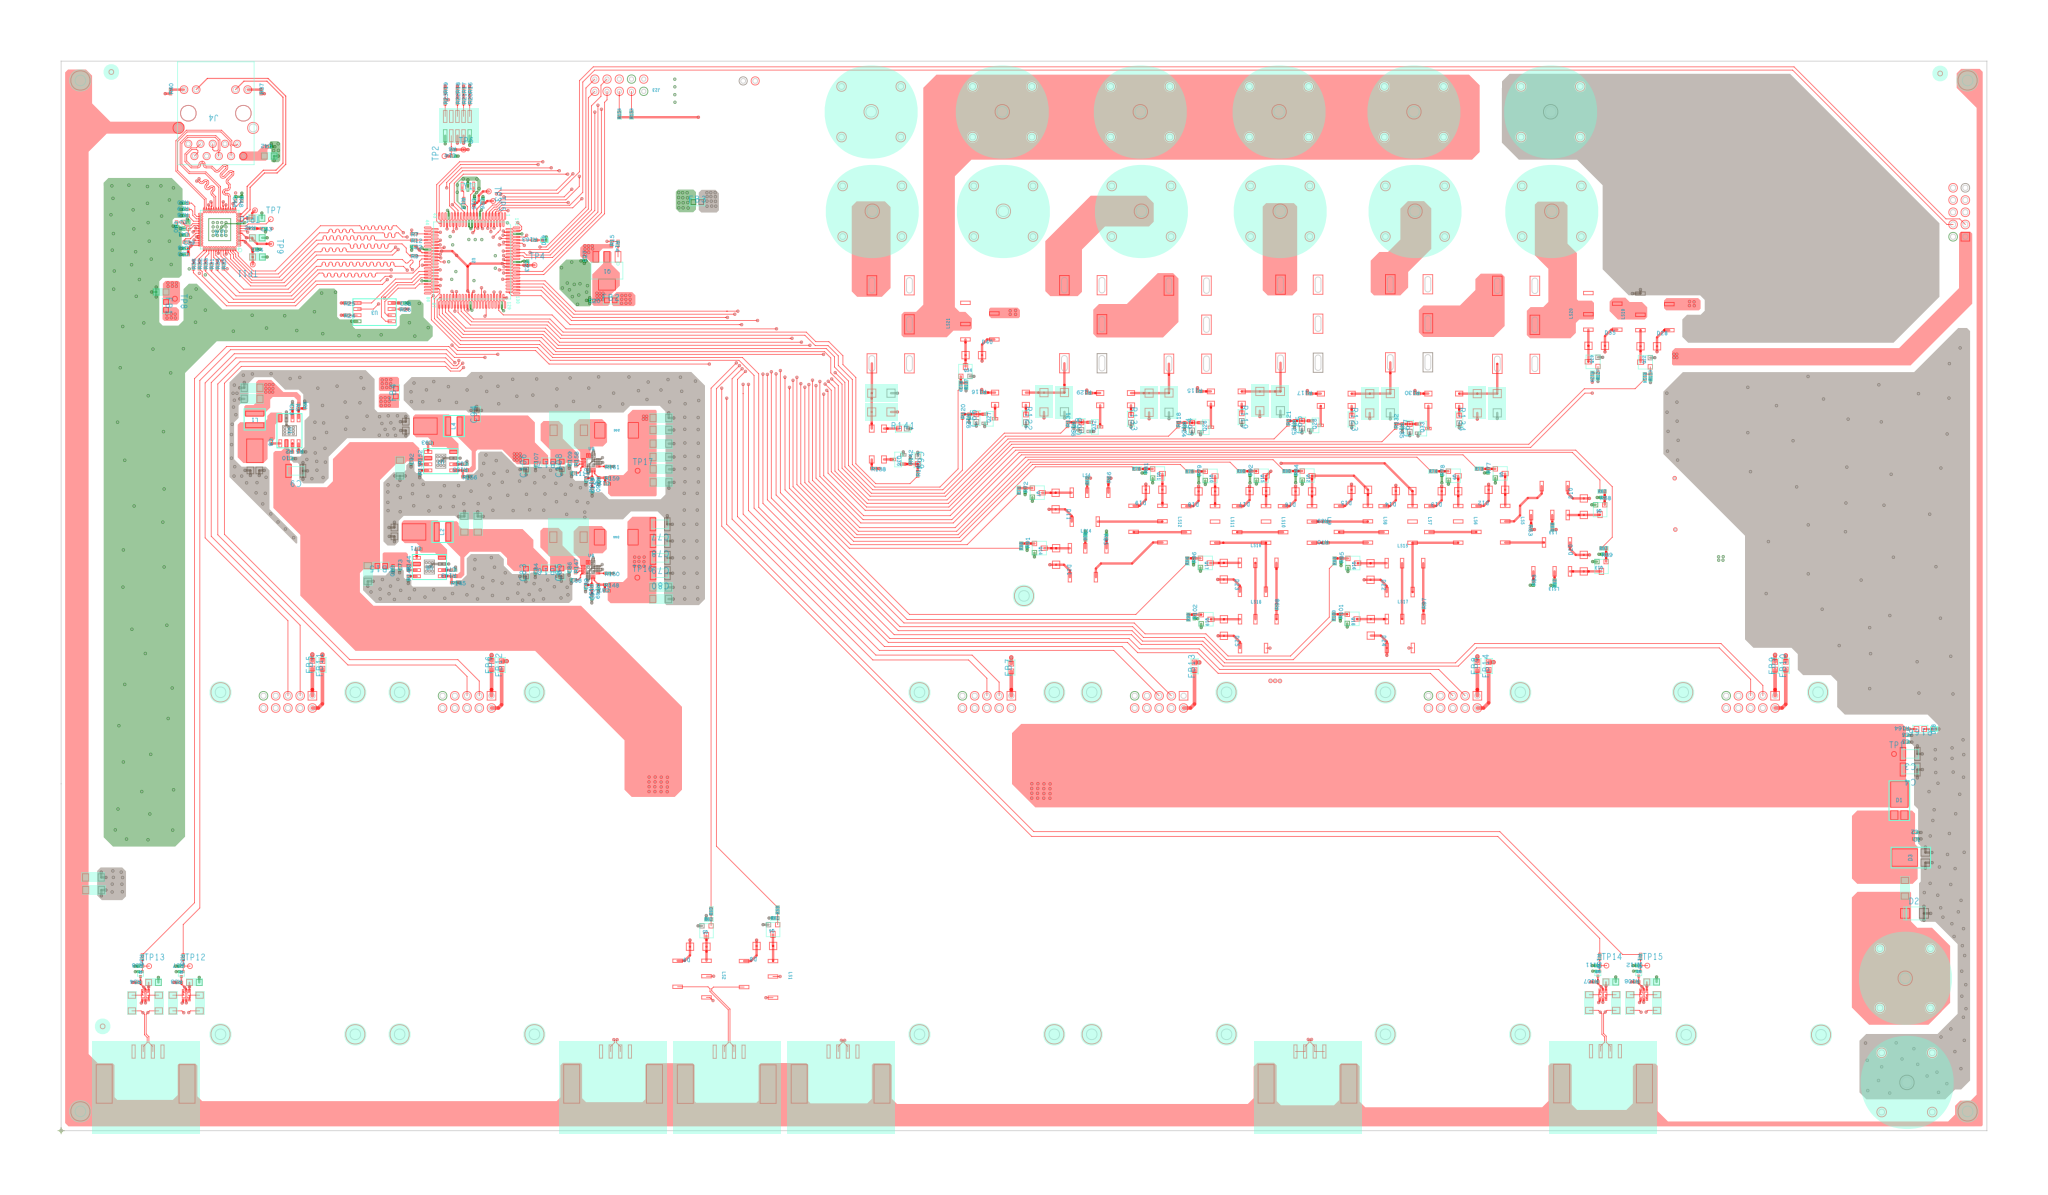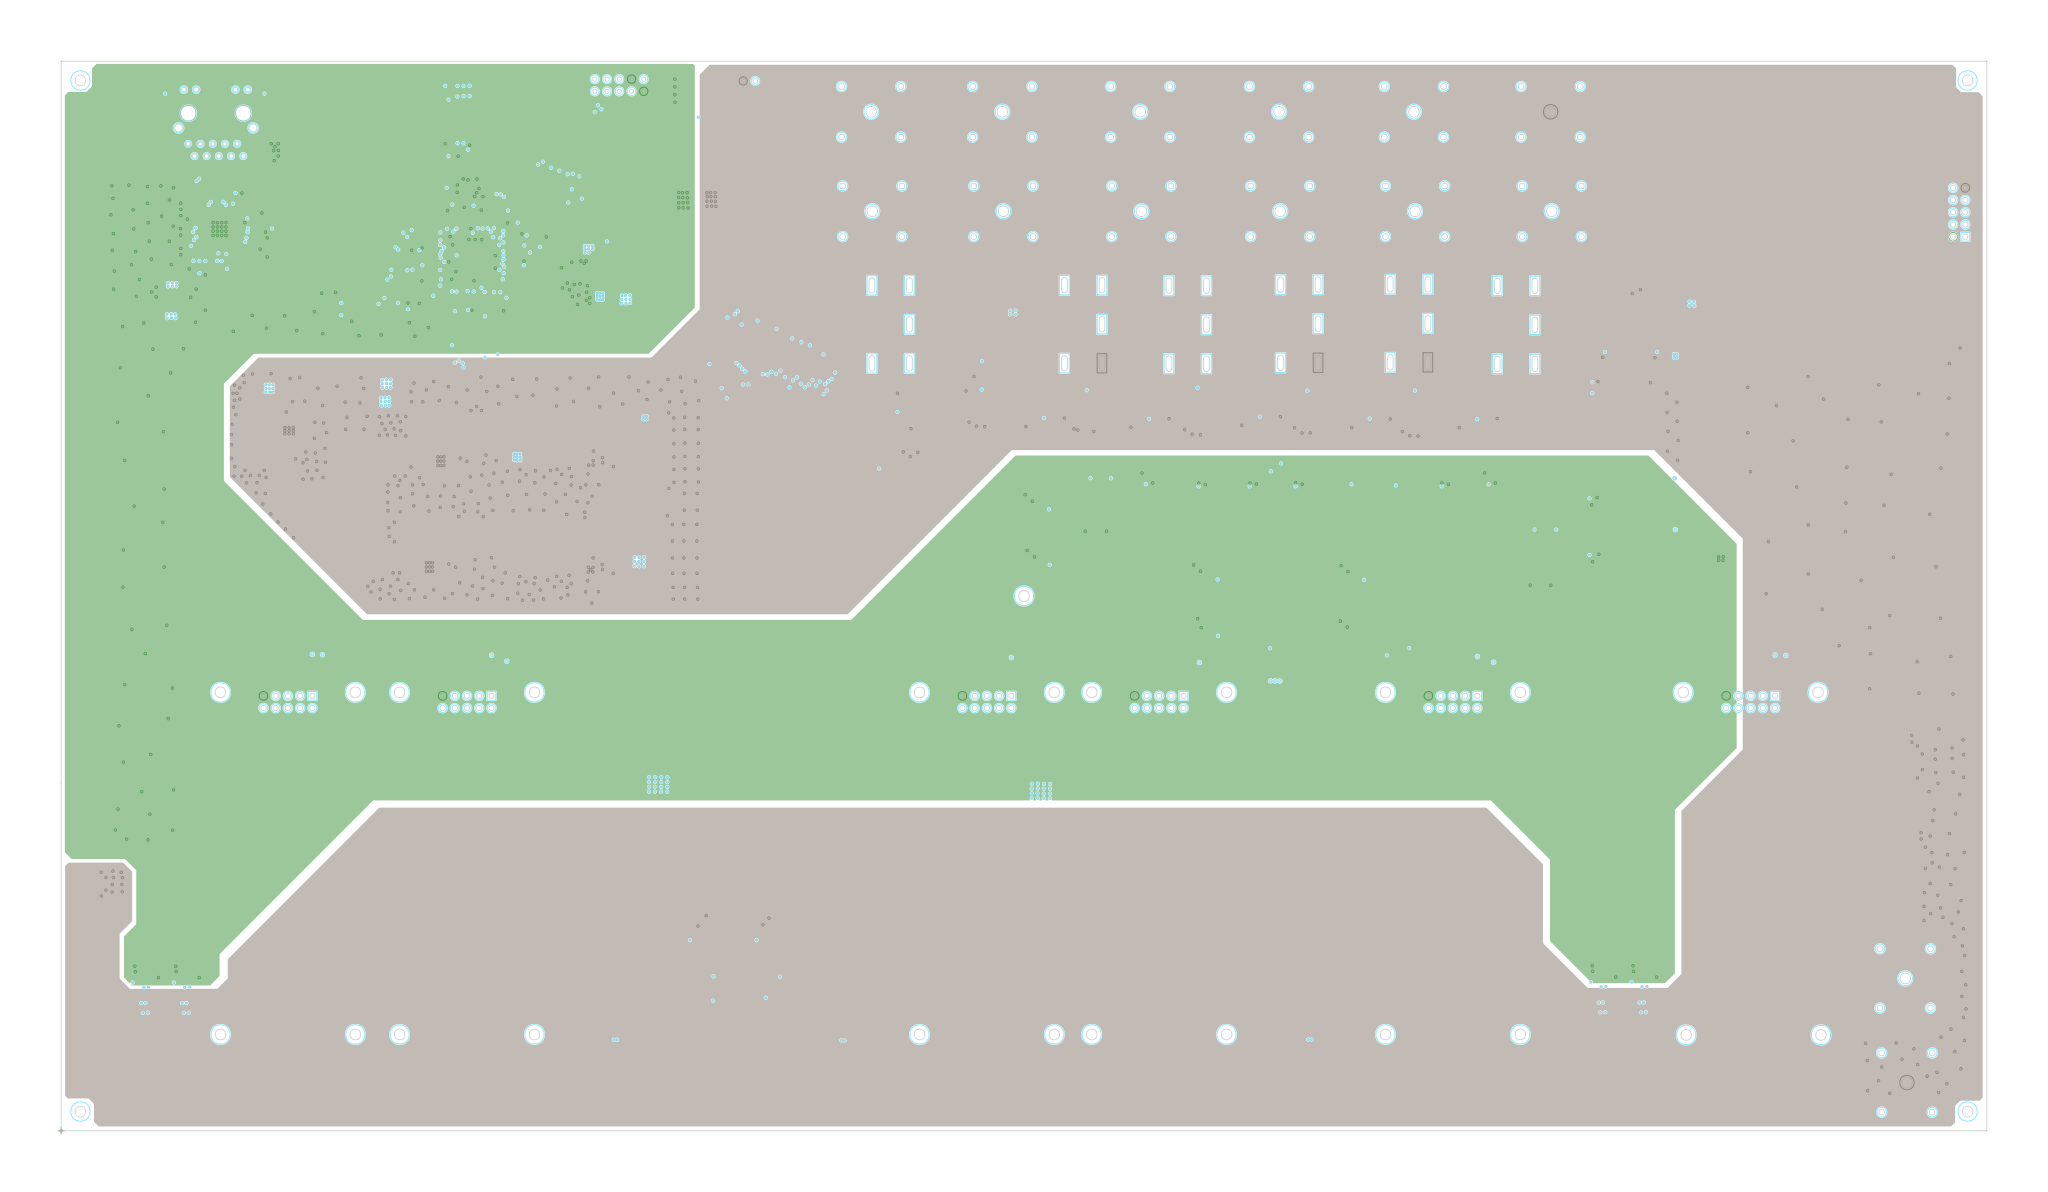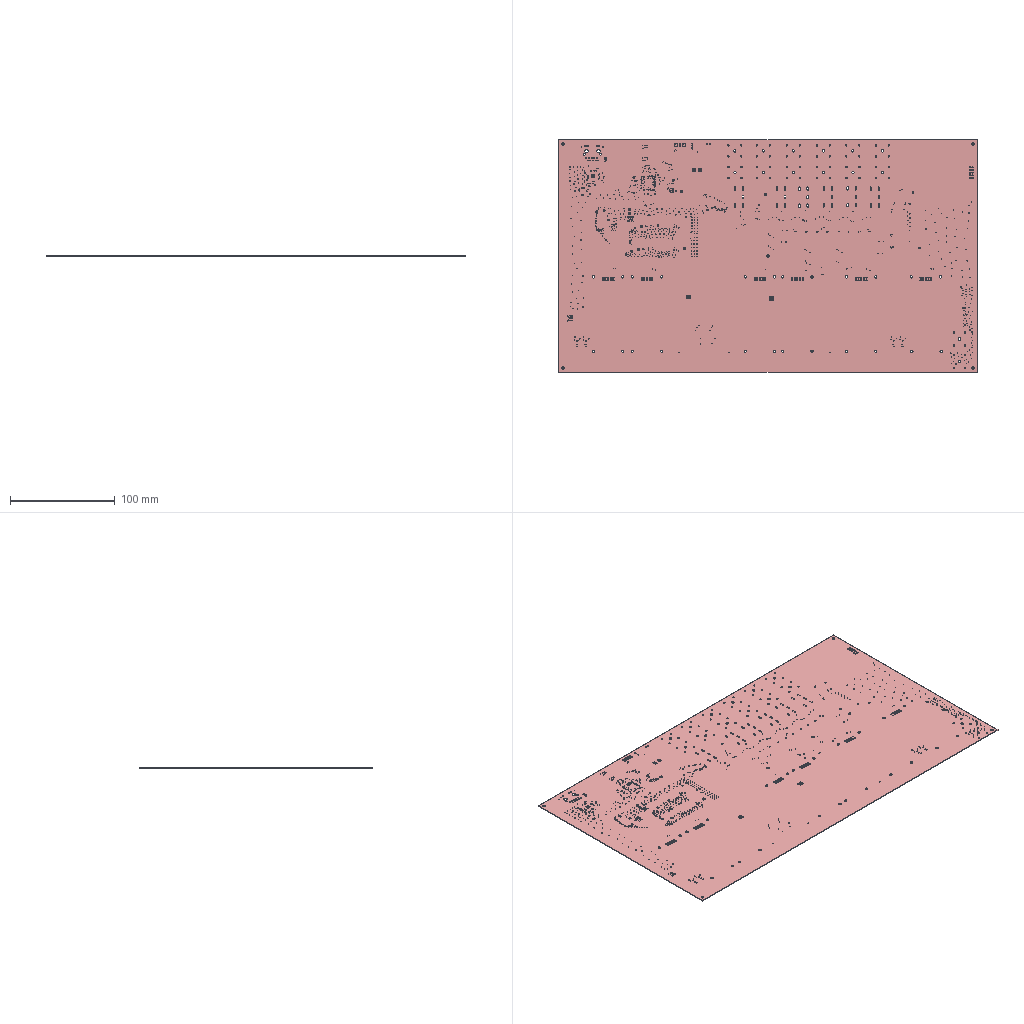Circuit board layout | Cadence Allegro | box 400 x 222 x 0.7 mm
Layer stack:
# Cadence Allegro layer stack of  (unit mm; from the constraint file cross-section; dielectric type: 0 not recorded (Allegro does not mark core vs prepreg), 3 surface material)
index,name,kind,layer,copper_thickness_mm,dielectric_type,dielectric_thickness_mm,dielectric_material,dielectric_constant
0,Top Surface,other,,,,,,
1,TOP,copper,TOP,0.0305,,,,
2,Dielectric1,dielectric,,,0,0.2032,FR-4,4.5
3,GND,copper,GND,0.0305,,,,
4,Dielectric2,dielectric,,,0,0.2032,FR-4,4.5
5,POWER,copper,POWER,0.0305,,,,
6,Dielectric3,dielectric,,,0,0.2032,FR-4,4.5
7,BOTTOM,copper,BOTTOM,0.0305,,,,
8,Bottom Surface,other,,,,,,
# drill layer pairs: low layer,high layer
drill_pair,TOP,BOTTOM
Part placement:
REFDES,COMP_VALUE,SYM_NAME,SYM_X,SYM_Y,SYM_ROTATE,SYM_MIRROR
C1,0.1uF,0402,15166.367,2384.239,0.000,NO
C2,1nF,0402,15166.922,2436.818,180.000,NO
C3,10uF_50V,1210,15121.023,3078.893,180.000,NO
C4,10uF_50V,1210,15121.082,2951.196,180.000,NO
C5,0.1uF,0402,15093.020,3175.308,180.000,NO
C6,0.1uF,0402,15092.303,3230.529,180.000,NO
C7,1nF_2kv,1206,264.027,2069.329,180.000,NO
C8,0.1uF,0402,1719.920,5633.244,270.000,NO
C9,4.7uF_50V,1210,1918.656,5392.020,180.000,NO
C10,0.1uF,0402,1876.644,5491.548,180.000,NO
C11,100uF_6.3V,1206,1561.850,6070.996,180.000,NO
C12,100uF_6.3V,1206,1561.850,5980.248,180.000,NO
C13,470pF,0402,1891.803,5916.799,270.000,NO
C14,0.1uF,0402,3207.680,7964.386,180.000,NO
C15,0.1uF,0402,3380.408,7598.514,270.000,NO
C16,0.1uF,0402,3152.512,7135.882,0.000,YES
C17,10uF_6.3V,0402,3324.539,6901.500,90.000,YES
C18,0.1uF,0402,3567.315,7076.476,180.000,YES
C19,0.1uF,0402,3152.744,7187.449,0.000,YES
C20,2.2uF_10V,0402,4339.004,6785.480,0.000,NO
C21,10uF_6.3V,0402,3335.079,6748.189,0.000,YES
C22,0.1uF,0402,2882.858,7226.445,0.000,NO
C23,0.1uF,0402,3814.416,7089.057,270.000,NO
C24,0.1uF,0402,3386.374,7322.535,270.000,YES
C25,0.1uF,0402,3333.787,7322.354,270.000,YES
C26,0.22uF_10V,0402,3449.655,7599.047,270.000,NO
C27,2.2uF_10V,0402,4278.176,7124.640,90.000,NO
C28,10uF 10V,0603,3168.937,7020.850,0.000,YES
C29,0.1uF,0402,3439.890,7324.008,270.000,YES
C30,0.1uF,0402,3627.398,7402.335,90.000,YES
C31,0.1uF,0402,3412.835,7432.705,90.000,YES
C32,0.1uF,0402,3153.031,7239.307,0.000,YES
C33,0.1uF,0402,3376.043,6902.587,90.000,YES
C34,0.1uF,0402,3567.205,7126.173,180.000,YES
C35,0.1uF,0402,3633.000,6763.000,270.000,YES
C36,0.1uF,0402,3153.795,6957.039,0.000,YES
C37,0.1uF,0402,3156.909,7323.500,270.000,YES
C38,0.1uF,0402,2792.173,6764.170,0.000,NO
C39,0.22uF,0402,1022.477,7261.467,0.000,NO
C40,6pF_1%,0402,943.650,7408.633,270.000,NO
C41,6pF_1%,0402,1022.803,7319.000,180.000,NO
C42,0.1uF,0402,1702.362,8041.280,180.000,NO
C43,47pF,0402,1654.564,7372.408,0.000,NO
C44,0.1uF,0402,1426.769,7614.459,270.000,NO
C45,0.1uF,0402,1443.836,7455.711,0.000,YES
C46,0.1uF,0402,1310.844,7507.601,90.000,YES
C47,0.1uF,0402,1237.922,7507.499,90.000,YES
C48,0.1uF,0402,1023.627,7208.982,180.000,NO
C49,0.1uF,0402,1155.950,7250.381,180.000,YES
C50,0.1uF,0402,1023.312,7159.380,180.000,NO
C51,0.1uF,0402,1287.103,7223.058,270.000,YES
C52,0.1uF,0402,1156.115,7347.444,180.000,YES
C53,0.1uF,0402,1345.635,7223.436,270.000,YES
C54,0.1uF,0402,1582.247,7203.564,0.000,NO
C55,0.1uF,0402,1436.119,7275.046,0.000,YES
C56,0.1uF,0402,1190.576,7507.830,90.000,YES
C57,0.1uF,0402,1156.576,7299.141,180.000,YES
C58,0.1uF,0402,1156.414,7396.361,180.000,YES
C59,0.1uF,0402,1359.395,7507.219,90.000,YES
C60,0.22uF 100V,0805,1089.356,1211.128,180.000,NO
C61,0.22uF 100V,0805,755.356,1211.128,180.000,NO
C62,0.22uF 100V,0805,12673.260,1215.236,180.000,NO
C63,0.22uF 100V,0805,13007.260,1215.236,180.000,NO
C64,2.2nF_50V,0603,9248.689,5753.737,90.000,NO
C65,2.2nF_50V,0603,10147.644,5769.551,90.000,NO
C66,2.2nF_50V,0603,7484.486,5823.367,90.000,NO
C67,2.2nF_50V,0603,11028.888,5743.297,90.000,NO
C68,2.2nF_50V,0603,8343.440,5757.279,90.000,NO
C69,2.2nF_50V,0603,7004.927,5479.234,270.000,NO
C70,1uF,0402,2714.401,4599.026,270.000,NO
C71,0.1uF,0402,2923.944,4752.892,180.000,NO
C72,10uF_50V,1206,2507.630,4553.368,90.000,NO
C73,0.1uF,0402,2768.099,4599.246,90.000,NO
C74,100uF_6.3V,1206,3406.840,4955.664,90.000,NO
C75,100uF_6.3V,1206,3297.656,4955.664,90.000,NO
C76,470pF,0402,3208.872,4581.288,180.000,NO
C77,4.7uF_50V,1210,4898.112,4955.552,180.000,NO
C78,4.7uF_50V,1210,4898.984,4818.957,180.000,NO
C79,4.7uF_50V,1210,4899.236,4681.124,180.000,NO
C80,4.7uF_50V,1210,4899.661,4555.730,180.000,NO
C81,10uF_50V,1206,4902.753,4439.805,180.000,NO
C82,10uF_50V,1206,4902.745,4344.734,180.000,NO
C83,10uF_16V,0603,3800.648,4560.868,90.000,NO
C84,0.1uF,0402,3877.016,4567.308,90.000,NO
C85,10uF_16V,0603,4090.788,4562.712,90.000,NO
C86,0.1uF,0402,4153.354,4577.976,90.000,NO
C87,20pF_25V,0402,4463.125,4411.714,180.000,NO
C88,47nF_10V,0402,4187.496,4501.654,0.000,NO
C89,100pF_16V,0402,4288.543,4443.821,90.000,NO
C90,0.1uF,0402,4339.653,4357.482,90.000,NO
C91,4.7uF_50V,1206,2770.610,5414.732,90.000,NO
C92,0.1uF,0402,2861.335,5464.146,90.000,NO
C93,0.1uF,0402,3017.180,5617.792,180.000,NO
C94,10uF_16V,0603,3398.560,5854.548,90.000,NO
C95,470pF,0402,3302.108,5446.188,180.000,NO
C96,10uF/25V,C0603,4955.605,8404.371,180.000,YES
C97,10uF/25V,C0603,4955.156,8466.548,180.000,YES
C98,10uF/25V,C0603,4955.416,8530.662,180.000,YES
C99,10uF/25V,C0603,4955.935,8592.840,180.000,YES
C100,4.7uF_50V,1206,4904.544,5614.512,180.000,NO
C101,4.7uF_50V,1206,4905.772,5404.728,180.000,NO
C102,4.7uF_50V,1206,4905.772,5297.996,180.000,NO
C103,4.7uF_50V,1206,4904.544,5824.300,180.000,NO
C104,10uF_50V,1206,4904.544,5726.152,180.000,NO
C105,10uF_50V,1206,4904.544,5505.328,180.000,NO
C106,10uF_16V,0603,3803.096,5434.360,90.000,NO
C107,0.1uF,0402,3879.464,5440.800,90.000,NO
C108,10uF_16V,0603,4093.236,5436.204,90.000,NO
C109,0.1uF,0402,4155.802,5451.468,90.000,NO
C110,20pF_25V,0402,4465.573,5285.206,180.000,NO
C111,47nF_10V,0402,4189.944,5375.146,0.000,NO
C112,100pF_16V,0402,4290.991,5317.313,90.000,NO
C113,0.1uF,0402,4342.101,5230.974,90.000,NO
CB1,22uF_10V,0805,1701.835,7964.729,0.000,NO
CB2,22uF_10V,0805,817.585,6853.851,180.000,NO
CB3,22uF_10V,0805,1603.878,7296.944,0.000,NO
CB4,22uF_10V,0805,1601.504,7456.003,0.000,NO
CB5,22uF_10V,0805,1605.773,7139.886,0.000,NO
D1,SL1045,TO277_65X40_H120,15032.464,2697.240,0.000,NO
D2,SMAJ36CA,SMAJ36,15156.630,1775.495,0.000,NO
D3,SL1045,TO277_65X40_H120,15126.394,2231.633,90.000,NO
D4,PDS760-13,PDS760,1584.004,5475.913,270.000,NO
D6,CSD87502Q2,DFN-6_2X2,1023.717,1107.114,0.000,NO
D7,CSD87502Q2,DFN-6_2X2,689.717,1107.114,0.000,NO
D8,DL4148,MINIMELF,5822.295,1509.303,180.000,NO
D9,DL4148,MINIMELF,5277.642,1503.358,180.000,NO
D10,DL4148,MINIMELF,12452.219,5031.852,90.000,NO
D11,DL4148,MINIMELF,8132.712,5212.978,270.000,NO
D12,DL4148,MINIMELF,11808.637,5237.525,180.000,NO
D13,DL4148,MINIMELF,11425.105,5225.482,180.000,NO
D14,DL4148,MINIMELF,11050.042,5226.998,180.000,NO
D15,DL4148,MINIMELF,10687.282,5237.297,180.000,NO
D16,DL4148,MINIMELF,10229.664,5224.022,180.000,NO
D17,DL4148,MINIMELF,9853.951,5226.352,180.000,NO
D18,DL4148,MINIMELF,9436.778,5224.337,180.000,NO
D19,DL4148,MINIMELF,9005.653,5238.073,180.000,NO
D20,DL4148,MINIMELF,12451.751,4570.325,90.000,NO
D21,DL4148,MINIMELF,8136.566,4759.915,270.000,NO
D22,DL4148,MINIMELF,10707.999,4637.018,270.000,NO
D23,DL4148,MINIMELF,9507.692,4639.569,270.000,NO
D24,DL4148,MINIMELF,10710.053,4180.729,270.000,NO
D25,DL4148,MINIMELF,9508.715,4179.032,270.000,NO
D26,CSD87502Q2,DFN-6_2X2,12607.621,1111.222,0.000,NO
D27,CSD87502Q2,DFN-6_2X2,12941.621,1111.222,0.000,NO
D28,DL4148,MINIMELF,12915.801,6410.084,0.000,NO
D29,SMAJ16A,DO-214AC,9970.841,5962.570,90.000,NO
D30,SMAJ16A,DO-214AC,9802.731,5962.300,270.000,NO
D31,SMAJ16A,DO-214AC,8205.008,5953.394,90.000,NO
D32,SMAJ16A,DO-214AC,8037.507,5952.516,270.000,NO
D33,SMAJ16A,DO-214AC,10869.900,5944.831,90.000,NO
D34,SMAJ16A,DO-214AC,10701.790,5943.953,270.000,NO
D35,DL4148,MINIMELF,12490.078,6414.102,0.000,NO
D36,SMAJ16A,DO-214AC,9059.747,5949.575,90.000,NO
D37,SMAJ16A,DO-214AC,8897.082,5948.698,270.000,NO
D38,SMAJ16A,DO-214AC,11744.154,5944.629,90.000,NO
D39,SMAJ16A,DO-214AC,11580.889,5944.359,270.000,NO
D40,DL4148,MINIMELF,7396.079,6337.715,0.000,NO
D41,SMAJ16A,DO-214AC,6707.776,6026.964,180.000,NO
D42,SMAJ16A,DO-214AC,6707.179,5873.400,0.000,NO
D43,PDS760-13,PDS760,2805.583,4892.934,180.000,NO
D44,B540C-13-F,SMC,4539.783,4849.992,180.000,NO
D45,PDS760-13,PDS760,2898.819,5757.834,180.000,NO
D46,B540C-13-F,SMC,4542.231,5723.484,180.000,NO
D48,NCD0402R1,LED0402_H050,15316.437,3282.242,90.000,NO
D49,NCD0402G1,LED0402_H050,3951.797,7277.576,90.000,NO
F1,Fuse_5A,1206,15077.756,1980.860,90.000,NO
FB1,BLM18KG300TN1D,0603,857.870,6740.076,270.000,NO
FB2,BLM18KG300TN1D,0603,4494.897,6785.278,0.000,NO
FB3,BLM18KG300TN1D,0603,5202.406,7588.192,0.000,NO
FB4,BLM18KG300TN1D,0603,2736.804,6032.536,90.000,NO
FB5,BLM18KG300TN1D,0603,2054.449,3807.862,90.000,NO
FB6,BLM18KG300TN1D,0603,3520.103,3805.863,90.000,NO
FB7,BLM18KG300TN1D,0603,7770.126,3784.850,90.000,NO
FB8,BLM18KG300TN1D,0603,11581.861,3797.677,90.000,NO
FB9,BLM18KG300TN1D,0603,14016.188,3799.077,90.000,NO
FB10,BLM18KG300TN1D,0603,14103.578,3799.739,90.000,NO
FB11,BLM18KG300TN1D,0603,2136.902,3806.469,90.000,NO
FB12,BLM18KG300TN1D,0603,3602.449,3805.256,90.000,NO
FB13,BLM18KG300TN1D,0603,9268.598,3795.001,90.000,NO
FB14,BLM18KG300TN1D,0603,11674.222,3796.973,90.000,NO
FB15,BLM18KG300TN1D,0603,2618.169,4615.868,180.000,NO
FB16,BLM18KG300TN1D,0603,3990.028,4594.500,180.000,NO
FB17,BLM18KG300TN1D,0603,3992.476,5467.992,180.000,NO
J1,4mm_Angled_Socket,YJX40016A,15080.346,1245.134,90.000,NO
J2,4mm_Angled_Socket,YJX40016A,15094.453,394.134,90.000,NO
J3,HB-PH9-12725PB2GOB,JTAG_2X5_1P27MM,3240.811,8209.965,180.000,NO
J4,HR915330AE,HR915330AE,1265.142,8314.736,180.000,NO
J5,BH254V-10P,BH254V-10P,1854.654,3503.909,180.000,NO
J6,4mm_Angled_Socket,YJX40016A,8825.083,8326.665,0.000,NO
J7,4mm_Angled_Socket,YJX40016A,8834.205,7513.695,0.000,NO
J8,BH254V-10P,BH254V-10P,3319.386,3503.909,180.000,NO
J9,349128040,349128040,4513.622,514.280,0.000,NO
J10,349128040,349128040,6374.303,514.280,0.000,NO
J11,349128040,349128040,5443.059,512.760,0.000,NO
J12,BH254V-10P,BH254V-10P,7570.622,3503.913,180.000,NO
J13,BH254V-10P,BH254V-10P,8979.106,3503.909,180.000,NO
J14,349128040,349128040,10192.319,514.567,0.000,NO
J15,4mm_Angled_Socket,YJX40016A,9960.028,8326.665,0.000,NO
J16,4mm_Angled_Socket,YJX40016A,9969.150,7513.691,0.000,NO
J17,4mm_Angled_Socket,YJX40016A,6633.248,7513.695,0.000,NO
J18,4mm_Angled_Socket,YJX40016A,6624.130,8326.661,0.000,NO
J19,BH254V-10P,BH254V-10P,11381.370,3503.909,180.000,NO
J20,4mm_Angled_Socket,YJX40016A,12189.957,7513.695,0.000,NO
J21,4mm_Angled_Socket,YJX40016A,12180.835,8326.665,0.000,NO
J22,B2B-XH-A,B2B-XH-A,5626.740,8578.846,0.000,NO
J23,BH2x5P_2.54,BH2X5P_2_54,4564.335,8543.811,180.000,NO
J25,BH254V-10P,BH254V-10P,15521.988,7505.402,90.000,NO
J26,4mm_Angled_Socket,YJX40016A,11062.811,8326.665,0.000,NO
J27,4mm_Angled_Socket,YJX40016A,11071.933,7513.695,0.000,NO
J28,4mm_Angled_Socket,YJX40016A,7696.409,8326.665,0.000,NO
J29,4mm_Angled_Socket,YJX40016A,7705.535,7513.691,0.000,NO
J30,BH254V-10P,BH254V-10P,13816.256,3504.157,180.000,NO
J31,349128040,349128040,690.921,513.929,0.000,NO
J32,349128040,349128040,12609.244,516.886,0.000,NO
L1,FEXL0430A-2R2M,L_41X41_H210_BOURNS,1583.098,5812.295,180.000,NO
L2,FEXL0430A-2R2M,L_41X41_H210_BOURNS,3119.072,4893.178,90.000,NO
L3,SLF7045T100M,SMD_7X7,4148.803,4850.437,0.000,NO
L4,FEXL0430A-2R2M,L_41X41_H210_BOURNS,3212.308,5758.078,90.000,NO
L5,SLF7045T100M,SMD_7X7,4151.251,5723.929,0.000,NO
LS1,IMC03GR,IMC03GR,5585.075,1385.996,270.000,NO
LS2,IMC03GR,IMC03GR,5041.327,1388.331,270.000,NO
LS3,IMC03GR,IMC03GR,12320.353,5267.360,180.000,NO
LS4,IMC03GR,IMC03GR,8264.574,4977.470,0.000,NO
LS5,IMC03GR,IMC03GR,11573.129,5105.663,270.000,NO
LS6,IMC03GR,IMC03GR,11188.653,5104.675,270.000,NO
LS7,IMC03GR,IMC03GR,10815.278,5103.793,270.000,NO
LS8,IMC03GR,IMC03GR,10449.810,5105.474,270.000,NO
LS9,IMC03GR,IMC03GR,9993.027,5103.514,270.000,NO
LS10,IMC03GR,IMC03GR,9617.235,5103.825,270.000,NO
LS11,IMC03GR,IMC03GR,9200.322,5103.529,270.000,NO
LS12,IMC03GR,IMC03GR,8770.145,5106.207,270.000,NO
LS13,IMC03GR,IMC03GR,12339.038,4806.951,180.000,NO
LS14,IMC03GR,IMC03GR,8249.278,4523.289,0.000,NO
LS15,IMC03GR,IMC03GR,10839.861,4401.510,0.000,NO
LS16,IMC03GR,IMC03GR,9639.554,4404.061,0.000,NO
LS17,IMC03GR,IMC03GR,10841.312,3944.617,0.000,NO
LS18,IMC03GR,IMC03GR,9640.582,3943.524,0.000,NO
LS19,IMC03GR,IMC03GR,13151.305,6541.950,90.000,NO
LS20,IMC03GR,IMC03GR,12725.582,6545.968,90.000,NO
LS21,IMC03GR,IMC03GR,7631.476,6466.035,90.000,NO
MH1,MOUNTING_HOLE,HOLE2_2_4,15590.551,157.480,0.000,NO
MH2,MOUNTING_HOLE,HOLE2_2_4,15590.551,8582.677,0.000,NO
MH3,MOUNTING_HOLE,HOLE2_2_4,157.480,8582.677,0.000,NO
MH4,MOUNTING_HOLE,HOLE2_2_4,157.480,157.480,0.000,NO
Q1,BCP56-16TX,BCP56_SOT-223,4463.479,7028.459,180.000,NO
Q2,CJ3134K KF,SOT723,982.913,1279.720,180.000,NO
Q3,CJ3134K KF,SOT723,648.913,1279.720,180.000,NO
Q4,NDS331N,SOT23-3,5859.484,1683.398,180.000,NO
Q5,NDS331N,SOT23-3,5315.217,1673.791,180.000,NO
Q6,NDS331N,SOT23-3,12623.058,5115.033,180.000,NO
Q7,NDS331N,SOT23-3,7942.499,5251.514,270.000,NO
Q8,NDS331N,SOT23-3,11728.496,5408.368,270.000,NO
Q9,NDS331N,SOT23-3,11344.920,5389.199,270.000,NO
Q10,NDS331N,SOT23-3,9356.590,5388.053,270.000,NO
Q11,NDS331N,SOT23-3,8926.119,5407.695,270.000,NO
Q12,NDS331N,SOT23-3,10149.223,5390.561,270.000,NO
Q13,NDS331N,SOT23-3,12634.428,4650.640,180.000,NO
Q14,NDS331N,SOT23-3,7959.507,4798.399,270.000,NO
Q15,NDS331N,SOT23-3,9774.514,5388.915,270.000,NO
Q16,NDS331N,SOT23-3,10522.987,4676.372,270.000,NO
Q17,NDS331N,SOT23-3,9317.095,4677.200,270.000,NO
Q18,NDS331N,SOT23-3,10517.317,4220.043,270.000,NO
Q19,NDS331N,SOT23-3,9323.222,4216.835,270.000,NO
Q20,CJ3134K KF,SOT723,12566.817,1283.828,180.000,NO
Q21,CJ3134K KF,SOT723,12900.817,1283.828,180.000,NO
Q22,NDS331N,SOT23-3,12995.823,6242.406,90.000,NO
Q23,TLP187,TLP187,9528.613,5991.528,270.000,NO
Q24,TLP187,TLP187,7763.389,5981.745,270.000,NO
Q25,TLP187,TLP187,10427.672,5973.186,270.000,NO
Q26,BSS138,003_SOT23B,9317.526,5786.151,0.000,NO
Q27,BSS138,003_SOT23B,7552.218,5855.229,0.000,NO
Q28,BSS138,003_SOT23B,10215.372,5801.409,0.000,NO
Q29,NDS331N,SOT23-3,12567.995,6245.367,90.000,NO
Q30,TLP187,TLP187,8622.960,5977.922,270.000,NO
Q31,TLP187,TLP187,11306.771,5973.587,270.000,NO
Q32,BSS138,003_SOT23B,8411.172,5789.137,0.000,NO
Q33,BSS138,003_SOT23B,11096.616,5775.159,0.000,NO
Q34,NDS331N,SOT23-3,7357.592,6164.352,0.000,NO
Q35,TLP187,TLP187,6678.996,5611.430,0.000,NO
Q36,BSS138,003_SOT23B,6886.936,5447.585,180.000,NO
R1,1M,1206,264.991,1966.310,0.000,NO
R2,100K,0402,1875.106,5545.811,180.000,NO
R3,51K,0402,1941.669,5918.819,270.000,NO
R4,15K,0402,1991.559,5918.898,90.000,NO
R5,20K,0402,1958.909,5546.988,180.000,NO
R6,4.7K,0402,3207.434,8017.034,180.000,NO
R7,33R,0402,2883.035,7329.154,0.000,NO
R8,33R,0402,2883.000,7328.744,180.000,YES
R9,33R,0402,2882.492,7150.524,0.000,NO
R10,33R,0402,2884.272,7226.547,180.000,YES
R11,33R,0402,2882.138,7276.886,180.000,YES
R12,33R,0402,2883.201,7277.307,0.000,NO
R13,0R,0402,3292.260,7600.390,270.000,NO
R14,10K,0402,4554.378,7250.672,270.000,NO
R15,2.2K,0402,4500.280,7251.105,90.000,NO
R16,4.7K,0402,3340.905,8498.590,90.000,NO
R17,4.7K,0402,3291.038,8498.717,90.000,NO
R18,4.7K,0402,3240.439,8499.024,90.000,NO
R19,4.7K,0402,3140.528,8498.881,90.000,NO
R20,33R,0402,3340.884,8410.028,90.000,NO
R21,33R,0402,3291.335,8410.146,90.000,NO
R22,33R,0402,3240.626,8409.941,90.000,NO
R23,33R,0402,3140.496,8408.717,90.000,NO
R24,4.7K,0402,2334.673,6664.475,0.000,NO
R25,4.7K,0402,2334.482,6764.138,0.000,NO
R26,10K,0402,2791.985,6714.205,0.000,NO
R28,49R9,0402,1020.036,7477.723,180.000,NO
R29,49R9,0402,1020.202,7528.956,180.000,NO
R30,4.99K,0402,1020.583,7580.066,180.000,NO
R31,33R,0402,1227.553,7060.363,90.000,NO
R32,33R,0402,1130.313,7060.422,90.000,NO
R33,33R,0402,1179.400,7060.682,90.000,NO
R34,33R,0402,1276.837,7060.607,90.000,NO
R35,33R,0402,1326.474,7060.576,90.000,NO
R36,33R,0402,1081.679,7059.190,90.000,NO
R37,510R,0402,1635.395,8490.854,90.000,NO
R38,4.7K,0402,1568.780,7318.235,180.000,YES
R39,4.7K,0402,1569.079,7372.668,180.000,YES
R40,510R,0402,894.325,8491.276,90.000,NO
R41,4.7K,0402,1426.773,7614.424,270.000,YES
R42,49R9,0402,1569.485,7372.570,180.000,NO
R43,4.7K,0402,1081.317,7059.182,270.000,YES
R44,4.7K,0402,1130.474,7060.154,270.000,YES
R45,4.7K,0402,1326.581,7060.257,270.000,YES
R46,4.7K,0402,1276.278,7060.650,270.000,YES
R47,4.7K,0402,1179.108,7060.871,270.000,YES
R48,4.7K,0402,1477.757,7615.255,270.000,NO
R49,49R9  0.4W 1206,1206,1132.583,1043.043,90.000,NO
R50,49R9  0.4W 1206,1206,912.640,1042.945,90.000,NO
R51,49R9  0.4W 1206,1206,798.583,1043.043,90.000,NO
R52,49R9  0.4W 1206,1206,578.640,1042.945,90.000,NO
R53,10K,0402,966.725,1211.525,180.000,NO
R54,10K,0402,632.725,1211.525,180.000,NO
R55,100R,0402,998.398,1419.035,270.000,NO
R56,100R,0402,664.398,1419.035,270.000,NO
R57,100R,0402,982.189,1344.772,180.000,NO
R58,100R,0402,648.189,1344.772,180.000,NO
R59,100R,R0402,5859.575,1804.209,90.000,NO
R60,100R,R0402,5314.965,1793.835,90.000,NO
R61,4.7K,R0402,5839.634,1737.697,0.000,NO
R62,4.7K,R0402,5295.445,1727.933,0.000,NO
R63,0R,0402,12021.161,4929.218,270.000,NO
R64,62R,R0402,12193.979,4932.179,270.000,NO
R65,62R,R0402,8390.948,5313.179,90.000,NO
R66,0R,0402,8564.554,5315.612,90.000,NO
R67,100R,R0402,12603.593,5224.651,0.000,NO
R68,4.7K,0402,12606.125,5174.466,0.000,NO
R69,1K,0402,10342.003,4977.475,180.000,NO
R70,0R,0402,10342.467,4804.407,180.000,NO
R71,100R,R0402,7832.881,5232.049,90.000,NO
R72,4.7K,0402,7883.066,5234.585,90.000,NO
R73,100R,R0402,11598.646,5408.041,0.000,NO
R74,100R,R0402,11221.754,5389.007,0.000,NO
R75,100R,R0402,9229.028,5387.262,0.000,NO
R76,100R,R0402,8794.369,5408.017,0.000,NO
R77,4.7K,0402,11668.748,5391.970,90.000,NO
R78,4.7K,0402,11291.070,5372.573,90.000,NO
R79,4.7K,0402,9302.739,5371.427,90.000,NO
R80,100R,R0402,10023.110,5390.606,0.000,NO
R81,4.7K,0402,8866.371,5391.298,90.000,NO
R82,62R,R0402,12213.184,4476.230,90.000,NO
R83,0R,0402,12039.562,4474.478,90.000,NO
R84,4.7K,0402,10095.281,5374.154,90.000,NO
R85,0R,0402,8548.751,4855.758,270.000,NO
R86,62R,R0402,8375.133,4854.006,270.000,NO
R87,100R,R0402,12614.528,4759.604,0.000,NO
R88,100R,R0402,7850.538,4779.111,90.000,NO
R89,4.7K,0402,12618.015,4710.722,0.000,NO
R90,100R,R0402,9651.812,5389.715,0.000,NO
R91,4.7K,0402,7899.424,4781.990,90.000,NO
R92,4.7K,0402,9722.104,5373.309,90.000,NO
R93,100R,R0402,10414.653,4657.417,90.000,NO
R94,100R,R0402,9208.577,4658.306,90.000,NO
R95,4.7K,0402,10466.570,4660.344,90.000,NO
R96,4.7K,0402,9260.677,4661.173,90.000,NO
R97,1K,0402,11140.799,4285.187,90.000,NO
R98,1K,0402,9938.912,4277.738,90.000,NO
R99,100R,R0402,9218.506,4197.280,90.000,NO
R100,100R,R0402,10408.191,4201.152,90.000,NO
R101,4.7K,0402,10460.904,4204.015,90.000,NO
R102,4.7K,0402,9266.805,4200.807,90.000,NO
R103,49R9  0.4W 1206,1206,12716.487,1047.151,90.000,NO
R104,49R9  0.4W 1206,1206,12496.544,1047.053,90.000,NO
R105,49R9  0.4W 1206,1206,13050.487,1047.151,90.000,NO
R106,49R9  0.4W 1206,1206,12830.544,1047.053,90.000,NO
R107,10K,0402,12550.629,1215.633,180.000,NO
R108,10K,0402,12884.629,1215.633,180.000,NO
R109,100R,0402,12582.302,1423.143,270.000,NO
R110,100R,0402,12916.302,1423.143,270.000,NO
R111,100R,0402,12566.093,1348.880,180.000,NO
R112,100R,0402,12900.093,1348.880,180.000,NO
R113,4.7K,R0402,12997.185,6162.670,90.000,NO
R114,100R,R0402,12951.488,6162.843,270.000,NO
R115,470R,0402,9309.205,6041.824,180.000,NO
R116,470R,0402,7544.996,6031.969,180.000,NO
R117,470R,0402,10207.724,6023.194,180.000,NO
R118,100R,0402,9132.945,5769.512,90.000,NO
R119,2k_0603,0603,9654.869,5831.016,270.000,NO
R120,100R,0402,7370.566,5838.838,90.000,NO
R121,100R,0402,10032.811,5784.110,90.000,NO
R122,2k_0603,0603,7889.645,5821.237,270.000,NO
R123,2k_0603,0603,10553.928,5812.674,270.000,NO
R124,4.7K,0402,9187.556,5769.572,270.000,NO
R125,4.7K,0402,10086.510,5784.473,270.000,NO
R126,4.7K,0402,7424.264,5838.593,270.000,NO
R127,4.7K,R0402,12567.868,6171.300,90.000,NO
R128,100R,R0402,12522.172,6171.477,270.000,NO
R129,470R,0402,8404.011,6027.930,180.000,NO
R130,470R,0402,11087.818,6023.711,180.000,NO
R131,100R,0402,8229.520,5772.446,90.000,NO
R132,100R,0402,10913.144,5758.768,90.000,NO
R133,2k_0603,0603,8749.216,5817.414,270.000,NO
R134,2k_0603,0603,11433.027,5813.075,270.000,NO
R135,4.7K,0402,10967.754,5758.523,270.000,NO
R136,4.7K,0402,8282.914,5772.506,270.000,NO
R137,4.7K,R0402,7400.025,6090.922,90.000,NO
R138,470R,0402,6645.516,5411.104,0.000,NO
R139,100R,R0402,7356.911,6091.222,270.000,NO
R140,100R,0402,7004.442,5366.944,90.000,NO
R141,2k_0603,0603,6883.972,5737.588,0.000,NO
R142,4.7K,0402,6943.361,5464.356,90.000,NO
R143,51.1K,0402,3209.024,4531.206,180.000,NO
R144,100K,0402,2837.764,4598.100,90.000,NO
R145,9.09K,0402,3209.811,4478.490,0.000,NO
R146,20K,0402,2838.630,4514.348,90.000,NO
R147,10K,0402,4206.496,4577.378,90.000,NO
R148,88.7K_1%,0402,4463.814,4461.785,0.000,NO
R149,10K,0402,4393.920,4445.884,270.000,NO
R150,78.7K_1%,0402,4467.036,4554.668,0.000,NO
R151,2.55K_1%,0402,4339.586,4443.899,270.000,NO
R152,100K,0402,2931.000,5463.000,90.000,NO
R153,NC,R0402,4663.897,8301.836,90.000,NO
R154,NC,R0402,4564.195,8302.122,90.000,NO
R155,51.1K,0402,3302.260,5396.106,180.000,NO
R156,9.09K,0402,3303.047,5343.390,0.000,NO
R157,20K,0402,2931.866,5379.248,90.000,NO
R158,10K_1%,0402,4208.944,5450.870,90.000,NO
R159,113K_1%,0402,4466.262,5335.277,0.000,NO
R160,10K_1%,0402,4396.368,5319.376,270.000,NO
R161,78.7K_1%,0402,4469.484,5428.160,0.000,NO
R162,2.55K_1%,0402,4342.034,5317.391,270.000,NO
R163,1.8K,0402,3870.315,7277.630,180.000,NO
R164,1.8K,0402,15092.597,3282.701,180.000,NO
R166,2k_0603,0603,15203.882,3282.513,180.000,NO
RY1,HFV9-012-1ZR,HFV9-012-1ZR,10125.361,6594.811,270.000,NO
RY2,HFV9-012-1ZR,HFV9-012-1ZR,8357.901,6590.520,270.000,NO
RY3,HFV9-012-1ZR,HFV9-012-1ZR,11023.161,6598.126,270.000,NO
RY4,HFV9-012-1ZR,HFV9-012-1ZR,9212.680,6586.929,270.000,NO
RY5,HFV9-012-1ZR,HFV9-012-1ZR,11898.141,6585.555,270.000,NO
RY6,HFV9-012-1ZR,HFV9-012-1ZR,6783.614,6589.531,270.000,NO
TP1,TP,S0400CI,14988.796,3078.372,0.000,NO
TP2,TP,S0400CI,3134.272,7964.144,90.000,NO
TP3,TP,S0400CI,3497.598,7675.665,270.000,NO
TP4,TP,S0400CI,3871.401,7073.045,0.000,NO
TP5,TP,S0400CI,3532.906,7597.425,270.000,NO
TP6,TP,S0400CI,3291.081,8017.433,0.000,NO
TP7,TP,S0400CI,1714.969,7448.700,0.000,NO
TP8,TP,S0400CI,930.452,6798.856,270.000,NO
TP9,TP,S0400CI,1717.928,7247.157,270.000,NO
TP10,TP,S0400CI,1585.260,7521.272,180.000,NO
TP11,TP,S0400CI,1566.969,7078.804,180.000,NO
TP12,TP,S0400CI,1053.614,1344.366,0.000,NO
TP13,TP,S0400CI,719.614,1344.366,0.000,NO
TP14,TP,S0400CI,12637.518,1348.474,0.000,NO
TP15,TP,S0400CI,12971.518,1348.474,0.000,NO
TP16,TP,S0400CI,4711.945,4519.469,0.000,NO
TP17,TP,S0400CI,4714.393,5392.961,0.000,NO
U1,LMR14050SQDDARQ1,SOP8P_60_PAD29X21_127_H170,1867.134,5719.744,270.000,NO
U2,S32K314EHTVBPBST_MaxQFP172,MQFP172_0P65_16X16,3360.819,7111.406,270.000,NO
U3,W25Q128JVSIQ,SO8P_79_127_H220,2563.090,6689.287,180.000,NO
U4,88EA1512_QFN56,QFN50P800X800X100-56N_180X180EP,1296.477,7363.239,180.000,NO
U5,LMR14050SQDDARQ1,SOP8P_60_PAD29X21_127_H170,3011.386,4606.124,180.000,NO
U6,TPS55340RTER,WQFN16-3X3,4270.826,4525.143,0.000,NO
U7,LMR14050SQDDARQ1,SOP8P_60_PAD29X21_127_H170,3104.622,5471.024,180.000,NO
U8,TPS55340RTER,WQFN16-3X3,4273.274,5398.635,0.000,NO
Y1,CSTNE16M0V53C000R0,CSTNE16M0V53C000R0,3326.374,7714.500,0.000,NO
Y2,XRCGB25M000F3A00R00,CRYSTAL_SM,1019.824,7398.826,90.000,NO
Pad and via stacks, first 112 of 394 lines:
# Allegro (Cadence) via spans and padstacks; design units: ("mils" 3 1000)
# via spans: padstack,start_layer,end_layer,net_example,count
VIA12X20,ETCH/TOP,ETCH/BOTTOM,BAT_GND,1173
VIA15_30,ETCH/TOP,ETCH/BOTTOM,NODE6_DUT_GND_PWR,15
# Allegro padstack definitions: name,start_layer,end_layer,drill,plating,holeType,type
PAD19,"ETCH/TOP","ETCH/TOP",0.0,"NON_PLATED","none","smd"
PAD13,"ETCH/TOP","ETCH/TOP",0.0,"NON_PLATED","none","smd"
PAD12,"ETCH/TOP","ETCH/TOP",0.0,"NON_PLATED","none","smd"
PAD17,"ETCH/TOP","ETCH/TOP",0.0,"NON_PLATED","none","smd"
PAD15,"ETCH/TOP","ETCH/TOP",0.0,"NON_PLATED","none","smd"
PAD16,"ETCH/TOP","ETCH/TOP",0.0,"NON_PLATED","none","smd"
PAD1,"ETCH/TOP","ETCH/TOP",0.0,"NON_PLATED","none","smd"
PAD46,"ETCH/TOP","ETCH/TOP",0.0,"NON_PLATED","none","smd"
PAD44,"ETCH/TOP","ETCH/TOP",0.0,"NON_PLATED","none","smd"
PAD8,"ETCH/TOP","ETCH/TOP",0.0,"NON_PLATED","none","smd"
PAD5,"ETCH/TOP","ETCH/TOP",0.0,"NON_PLATED","none","smd"
PAD9,"ETCH/TOP","ETCH/TOP",0.0,"NON_PLATED","none","smd"
PAD10,"ETCH/TOP","ETCH/TOP",0.0,"NON_PLATED","none","smd"
PAD25,"ETCH/TOP","ETCH/TOP",0.0,"NON_PLATED","none","smd"
PAD4,"ETCH/TOP","ETCH/TOP",0.0,"NON_PLATED","none","smd"
PAD7,"ETCH/TOP","ETCH/TOP",0.0,"NON_PLATED","none","smd"
PAD6,"ETCH/TOP","ETCH/TOP",0.0,"NON_PLATED","none","smd"
PAD3,"ETCH/TOP","ETCH/TOP",0.0,"NON_PLATED","none","smd"
PAD31,"ETCH/TOP","ETCH/TOP",0.0,"NON_PLATED","none","smd"
PAD22,"ETCH/TOP","ETCH/TOP",0.0,"NON_PLATED","none","smd"
PAD41,"ETCH/TOP","ETCH/TOP",0.0,"NON_PLATED","none","smd"
PAD42,"ETCH/TOP","ETCH/TOP",0.0,"NON_PLATED","none","smd"
PAD43,"ETCH/TOP","ETCH/TOP",0.0,"NON_PLATED","none","smd"
PAD45,"ETCH/TOP","ETCH/TOP",0.0,"NON_PLATED","none","smd"
PAD2,"ETCH/TOP","ETCH/TOP",0.0,"NON_PLATED","none","smd"
PAD14,"ETCH/TOP","ETCH/TOP",0.0,"NON_PLATED","none","smd"
PAD21,"ETCH/TOP","ETCH/TOP",0.0,"NON_PLATED","none","smd"
PAD28,"ETCH/TOP","ETCH/TOP",0.0,"NON_PLATED","none","smd"
PAD26,"ETCH/TOP","ETCH/TOP",0.0,"NON_PLATED","none","smd"
PAD27,"ETCH/TOP","ETCH/TOP",0.0,"NON_PLATED","none","smd"
PAD18,"ETCH/TOP","ETCH/TOP",0.0,"NON_PLATED","none","smd"
PAD29,"ETCH/TOP","ETCH/TOP",0.0,"NON_PLATED","none","smd"
PAD20,"ETCH/TOP","ETCH/TOP",0.0,"NON_PLATED","none","smd"
PAD39,"ETCH/TOP","ETCH/TOP",0.0,"NON_PLATED","none","smd"
PAD40,"ETCH/TOP","ETCH/TOP",0.0,"NON_PLATED","none","smd"
PAD30,"ETCH/TOP","ETCH/TOP",0.0,"NON_PLATED","none","smd"
PAD48,"ETCH/TOP","ETCH/TOP",0.0,"NON_PLATED","none","smd"
PAD47,"ETCH/TOP","ETCH/TOP",0.0,"NON_PLATED","none","smd"
PAD49,"ETCH/TOP","ETCH/TOP",0.0,"NON_PLATED","none","smd"
PAD50,"ETCH/TOP","ETCH/TOP",0.0,"NON_PLATED","none","smd"
PAD53,"ETCH/TOP","ETCH/TOP",0.0,"NON_PLATED","none","smd"
F45,"ETCH/TOP","ETCH/TOP",0.0,"NON_PLATED","none","smd"
R88X76,"ETCH/TOP","ETCH/TOP",0.0,"PLATED","none","smd"
R127X121,"ETCH/TOP","ETCH/TOP",0.0,"PLATED","none","smd"
R127X152,"ETCH/TOP","ETCH/TOP",0.0,"NON_PLATED","none","smd"
R14X25,"ETCH/TOP","ETCH/TOP",0.0,"NON_PLATED","none","smd"
R165X317,"ETCH/TOP","ETCH/TOP",0.0,"NON_PLATED","none","smd"
R259X218,"ETCH/TOP","ETCH/TOP",0.0,"NON_PLATED","none","smd"
R70X22,"ETCH/TOP","ETCH/TOP",0.0,"NON_PLATED","none","smd"
R75X85,"ETCH/TOP","ETCH/TOP",0.0,"NON_PLATED","none","smd"
Y5,"ETCH/TOP","ETCH/TOP",0.0,"NON_PLATED","none","smd"
R16X30,"ETCH/TOP","ETCH/TOP",0.0,"NON_PLATED","none","smd"
F62X58,"ETCH/TOP","ETCH/TOP",0.0,"PLATED","none","smd"
R15X28,"ETCH/TOP","ETCH/TOP",0.0,"NON_PLATED","none","smd"
R195X280,"ETCH/TOP","ETCH/TOP",0.0,"NON_PLATED","none","smd"
R45X200,"ETCH/TOP","ETCH/TOP",0.0,"NON_PLATED","none","smd"
R50X30,"ETCH/TOP","ETCH/TOP",0.0,"NON_PLATED","none","smd"
R127X120,"ETCH/TOP","ETCH/TOP",0.0,"NON_PLATED","none","smd"
R31X24,"ETCH/TOP","ETCH/TOP",0.0,"NON_PLATED","none","smd"
R215X60,"ETCH/TOP","ETCH/TOP",0.0,"NON_PLATED","none","smd"
S17,"ETCH/TOP","ETCH/TOP",0.0,"NON_PLATED","none","smd"
R23X25,"ETCH/TOP","ETCH/TOP",0.0,"NON_PLATED","none","smd"
R19X32,"ETCH/TOP","ETCH/TOP",0.0,"NON_PLATED","none","smd"
R61X15,"ETCH/TOP","ETCH/TOP",0.0,"NON_PLATED","none","smd"
R45X150,"ETCH/TOP","ETCH/TOP",0.0,"NON_PLATED","none","smd"
R12X8,"ETCH/TOP","ETCH/TOP",0.0,"NON_PLATED","none","smd"
R91X127,"ETCH/TOP","ETCH/TOP",0.0,"NON_PLATED","none","smd"
S91,"ETCH/TOP","ETCH/TOP",0.0,"NON_PLATED","none","smd"
R55X99,"ETCH/TOP","ETCH/TOP",0.0,"NON_PLATED","none","smd"
R299X199,"ETCH/TOP","ETCH/TOP",0.0,"NON_PLATED","none","smd"
R114X165,"ETCH/TOP","ETCH/TOP",0.0,"NON_PLATED","none","smd"
R60X90,"ETCH/TOP","ETCH/TOP",0.0,"NON_PLATED","none","smd"
R6X10,"ETCH/TOP","ETCH/TOP",0.0,"NON_PLATED","none","smd"
Y10,"ETCH/TOP","ETCH/TOP",0.0,"NON_PLATED","none","smd"
R114X74,"ETCH/TOP","ETCH/TOP",0.0,"NON_PLATED","none","smd"
R30X130,"ETCH/TOP","ETCH/TOP",0.0,"PLATED","none","smd"
R50X127,"ETCH/TOP","ETCH/TOP",0.0,"NON_PLATED","none","smd"
R18X20,"ETCH/TOP","ETCH/TOP",0.0,"NON_PLATED","none","smd"
R60X71,"ETCH/TOP","ETCH/TOP",0.0,"NON_PLATED","none","smd"
R48X71,"ETCH/TOP","ETCH/TOP",0.0,"NON_PLATED","none","smd"
R80X30,"ETCH/TOP","ETCH/TOP",0.0,"PLATED","none","smd"
FLASH_0,"ETCH/TOP","ETCH/TOP",0.0,"PLATED","none","smd"
Y3,"ETCH/TOP","ETCH/TOP",0.0,"PLATED","none","smd"
R170X25,"ETCH/TOP","ETCH/TOP",0.0,"PLATED","none","smd"
R70X25,"ETCH/TOP","ETCH/TOP",0.0,"PLATED","none","smd"
R43X14,"ETCH/TOP","ETCH/TOP",0.0,"PLATED","none","smd"
R33X10,"ETCH/TOP","ETCH/TOP",0.0,"PLATED","none","smd"
R636X23,"ETCH/TOP","ETCH/TOP",0.0,"PLATED","none","smd"
R155X35,"ETCH/TOP","ETCH/TOP",0.0,"PLATED","none","smd"
R60X20,"ETCH/TOP","ETCH/TOP",0.0,"PLATED","none","smd"
R120X70,"ETCH/TOP","ETCH/TOP",0.0,"PLATED","none","smd"
SMD0_45R,"ETCH/TOP","ETCH/TOP",0.0,"PLATED","none","smd"
Y42,"ETCH/TOP","ETCH/TOP",0.0,"PLATED","none","smd"
R85X65,"ETCH/TOP","ETCH/TOP",0.0,"PLATED","none","smd"
Y30,"ETCH/TOP","ETCH/TOP",0.0,"PLATED","none","smd"
R53X20,"ETCH/TOP","ETCH/TOP",0.0,"PLATED","none","smd"
R55X40,"ETCH/TOP","ETCH/TOP",0.0,"PLATED","none","smd"
R155X25,"ETCH/TOP","ETCH/TOP",0.0,"PLATED","none","smd"
F17X17,"ETCH/TOP","ETCH/TOP",0.0,"PLATED","none","smd"
F89X32,"ETCH/TOP","ETCH/TOP",0.0,"PLATED","none","smd"
R8X2,"ETCH/TOP","ETCH/TOP",0.0,"PLATED","none","smd"
SMD40X20,"ETCH/TOP","ETCH/TOP",0.0,"PLATED","none","smd"
R340X185,"ETCH/TOP","ETCH/TOP",0.0,"PLATED","none","smd"
R27X10,"ETCH/TOP","ETCH/TOP",0.0,"PLATED","none","smd"
R22X11,"ETCH/TOP","ETCH/TOP",0.0,"PLATED","none","smd"
R32X36,"ETCH/TOP","ETCH/TOP",0.0,"PLATED","none","smd"
S21X20,"ETCH/TOP","ETCH/TOP",0.0,"PLATED","none","smd"
Design rules, without the lines most boards share, first 10 of 39 lines:
# Cadence Allegro design rules of  (from the Constraint Manager export constraints.dcfx, design unit mil; typed fields in mm)
# columns: name | kind | enabled | priority | scope1 | scope2 | descriptor | typed fields (field=value)
# Allegro precedence (priority 1 wins): 1 Region class-to-class, 2 Region class, 3 Region, 4 class-to-class, 5 DiffPair/Bus/NetGroup override, 6 NetClass, 7 constraint set (CSet) default
# per-layer values are written LAYER=value in the descriptor and LAYER:mm in the typed field; a maximum of 0 means no limit set
# --- net classes (and buses / net groups) ---
PHY_TX | NetClass | enabled | 6 | MII_TX_CTRL_PTD11, MII_TXD2_PTD6, MII_TXD3_PTD5, MII_TXD0_PTB5, MII_TX_CLK_PTC0, MII_TXD1_PTB4 | All | Net Class (members: 6 Xnet) |
PHY_RX | NetClass | enabled | 6 | 1512_RX_CTRL, 1512_RXD[0], MII_RX_CLK_PTC1, 1512_RXD[2], 1512_RXD[1], 1512_RXD[3] | All | Net Class (members: 6 Xnet) |
PHY | NetClass | enabled | 6 | DIFFPAIR3, DIFFPAIR2, DIFFPAIR1, DIFFPAIR0 | All | Net Class (members: 4 DiffPair) |
# --- track widths, neck and differential-pair gap (physical constraint sets) ---
DEFAULT | PhysicalCSet | enabled | 7 | Design default | All | Physical Constraint (Min Line Width=7mil) (Max Line Width=0mil) (Min Neck Width=7mil) (Max Neck Length=0mil) (DiffPair Primary Gap=7mil) (DiffPair Neck Gap=0mil) (DiffPair Min Space=0mil) (DiffPair Coupled +Tol=0mil) (DiffPair Coupled -Tol=0mil) (Min BB Via Stagger=7mil) (Max BB Via Stagger=0mil) (T-junctions=ANYWHERE) (Pad-pad direct connect=ALL_ALLOWED) (Allowed vias=VIA12X20, VIA15_30) | min_line_width=0.1778 min_neck_width=0.1778 min_bvia_stagger=0.1778 max_bvia_stagger=0 ts_allowed=ANYWHERE diffp_primary_gap=0.1778 diffp_neck_gap=0 max_line_width=0 maximum_neck_length=0 pad_pad_direct_connect=ALL_ALLOWED allow_on_etch_subclass=TRUE diffp_coupled_plus=0 diffp_coupled_minus=0 diffp_min_space=0 vias=VIA12X20,VIA15_30